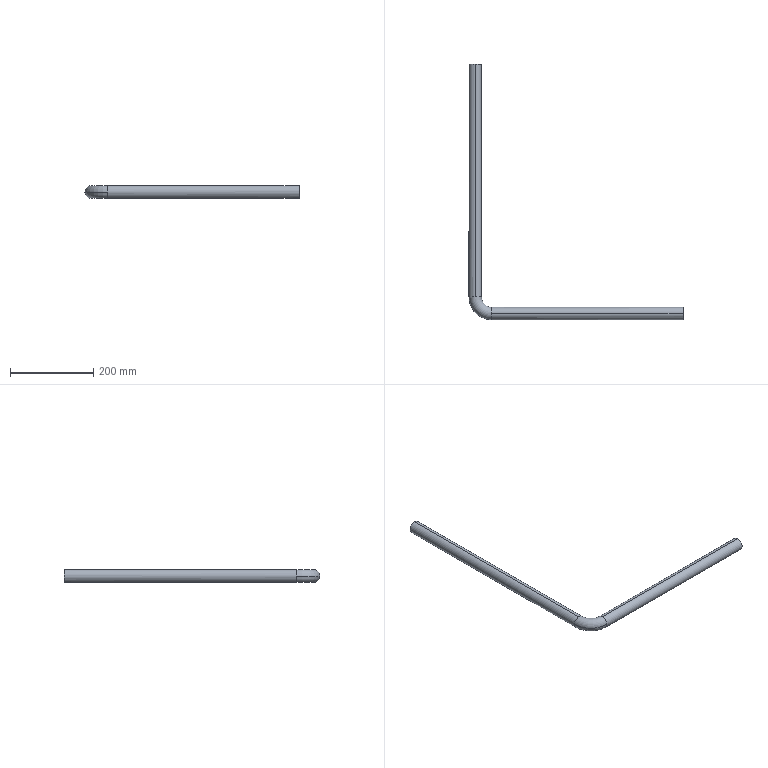Part | SolidWorks | features Sweep 1 | 1 solid | 14 faces | box 515 x 615 x 30 mm | volume 190502 mm3 | cylinder 8 | torus 4 | plane 2 | commonest cylinder face diameters 26 x4 30 x4
STEP:
#1=CARTESIAN_POINT('',(40.,0.,13.));
#2=VERTEX_POINT('',#1);
#3=CARTESIAN_POINT('',(40.,-13.,0.));
#4=VERTEX_POINT('',#3);
#5=CARTESIAN_POINT('',(40.,0.,0.));
#6=DIRECTION('',(1.,0.,0.));
#7=DIRECTION('',(0.,0.,1.));
#8=AXIS2_PLACEMENT_3D('',#5,#6,#7);
#9=CIRCLE('',#8,13.);
#10=EDGE_CURVE('',#2,#4,#9,.T.);
#11=ORIENTED_EDGE('',*,*,#10,.T.);
#12=CARTESIAN_POINT('',(-13.,40.,0.));
#13=VERTEX_POINT('',#12);
#14=CARTESIAN_POINT('',(40.,40.,0.));
#15=DIRECTION('',(0.,0.,-1.));
#16=DIRECTION('',(-1.,0.,0.));
#17=AXIS2_PLACEMENT_3D('',#14,#15,#16);
#18=CIRCLE('',#17,53.);
#19=EDGE_CURVE('',#4,#13,#18,.T.);
#20=ORIENTED_EDGE('',*,*,#19,.T.);
#21=CARTESIAN_POINT('',(0.,40.,13.));
#22=VERTEX_POINT('',#21);
#23=CARTESIAN_POINT('',(0.,40.,0.));
#24=DIRECTION('',(0.,-1.,0.));
#25=DIRECTION('',(1.,0.,0.));
#26=AXIS2_PLACEMENT_3D('',#23,#24,#25);
#27=CIRCLE('',#26,13.);
#28=EDGE_CURVE('',#22,#13,#27,.T.);
#29=ORIENTED_EDGE('',*,*,#28,.F.);
#30=CARTESIAN_POINT('',(13.,40.,0.));
#31=VERTEX_POINT('',#30);
#32=CARTESIAN_POINT('',(0.,40.,0.));
#33=DIRECTION('',(0.,-1.,0.));
#34=DIRECTION('',(1.,0.,0.));
#35=AXIS2_PLACEMENT_3D('',#32,#33,#34);
#36=CIRCLE('',#35,13.);
#37=EDGE_CURVE('',#31,#22,#36,.T.);
#38=ORIENTED_EDGE('',*,*,#37,.F.);
#39=CARTESIAN_POINT('',(40.,13.,0.));
#40=VERTEX_POINT('',#39);
#41=CARTESIAN_POINT('',(40.,40.,0.));
#42=DIRECTION('',(0.,0.,-1.));
#43=DIRECTION('',(-1.,0.,0.));
#44=AXIS2_PLACEMENT_3D('',#41,#42,#43);
#45=CIRCLE('',#44,27.);
#46=EDGE_CURVE('',#40,#31,#45,.T.);
#47=ORIENTED_EDGE('',*,*,#46,.F.);
#48=CARTESIAN_POINT('',(40.,0.,0.));
#49=DIRECTION('',(1.,0.,0.));
#50=DIRECTION('',(0.,0.,1.));
#51=AXIS2_PLACEMENT_3D('',#48,#49,#50);
#52=CIRCLE('',#51,13.);
#53=EDGE_CURVE('',#40,#2,#52,.T.);
#54=ORIENTED_EDGE('',*,*,#53,.T.);
#55=EDGE_LOOP('',(#11,#20,#29,#38,#47,#54));
#56=FACE_OUTER_BOUND('',#55,.T.);
#57=CARTESIAN_POINT('',(40.,40.,0.));
#58=DIRECTION('',(0.,0.,-1.));
#59=DIRECTION('',(-1.,0.,0.));
#60=AXIS2_PLACEMENT_3D('',#57,#58,#59);
#61=TOROIDAL_SURFACE('',#60,40.,13.);
#62=ADVANCED_FACE('',(#56),#61,.F.);
#63=CARTESIAN_POINT('',(40.,-15.,0.));
#64=VERTEX_POINT('',#63);
#65=CARTESIAN_POINT('',(40.,0.,-15.));
#66=VERTEX_POINT('',#65);
#67=CARTESIAN_POINT('',(40.,0.,0.));
#68=DIRECTION('',(1.,0.,0.));
#69=DIRECTION('',(0.,0.,-1.));
#70=AXIS2_PLACEMENT_3D('',#67,#68,#69);
#71=CIRCLE('',#70,15.);
#72=EDGE_CURVE('',#64,#66,#71,.T.);
#73=ORIENTED_EDGE('',*,*,#72,.F.);
#74=CARTESIAN_POINT('',(-15.,40.,0.));
#75=VERTEX_POINT('',#74);
#76=CARTESIAN_POINT('',(40.,40.,0.));
#77=DIRECTION('',(0.,0.,-1.));
#78=DIRECTION('',(-1.,0.,0.));
#79=AXIS2_PLACEMENT_3D('',#76,#77,#78);
#80=CIRCLE('',#79,55.);
#81=EDGE_CURVE('',#64,#75,#80,.T.);
#82=ORIENTED_EDGE('',*,*,#81,.T.);
#83=CARTESIAN_POINT('',(0.,40.,-15.));
#84=VERTEX_POINT('',#83);
#85=CARTESIAN_POINT('',(0.,40.,0.));
#86=DIRECTION('',(0.,-1.,0.));
#87=DIRECTION('',(0.,0.,-1.));
#88=AXIS2_PLACEMENT_3D('',#85,#86,#87);
#89=CIRCLE('',#88,15.);
#90=EDGE_CURVE('',#75,#84,#89,.T.);
#91=ORIENTED_EDGE('',*,*,#90,.T.);
#92=CARTESIAN_POINT('',(15.,40.,0.));
#93=VERTEX_POINT('',#92);
#94=CARTESIAN_POINT('',(0.,40.,0.));
#95=DIRECTION('',(0.,-1.,0.));
#96=DIRECTION('',(0.,0.,-1.));
#97=AXIS2_PLACEMENT_3D('',#94,#95,#96);
#98=CIRCLE('',#97,15.);
#99=EDGE_CURVE('',#84,#93,#98,.T.);
#100=ORIENTED_EDGE('',*,*,#99,.T.);
#101=CARTESIAN_POINT('',(40.,15.,0.));
#102=VERTEX_POINT('',#101);
#103=CARTESIAN_POINT('',(40.,40.,0.));
#104=DIRECTION('',(0.,0.,-1.));
#105=DIRECTION('',(-1.,0.,0.));
#106=AXIS2_PLACEMENT_3D('',#103,#104,#105);
#107=CIRCLE('',#106,25.);
#108=EDGE_CURVE('',#102,#93,#107,.T.);
#109=ORIENTED_EDGE('',*,*,#108,.F.);
#110=CARTESIAN_POINT('',(40.,0.,0.));
#111=DIRECTION('',(1.,0.,0.));
#112=DIRECTION('',(0.,0.,-1.));
#113=AXIS2_PLACEMENT_3D('',#110,#111,#112);
#114=CIRCLE('',#113,15.);
#115=EDGE_CURVE('',#66,#102,#114,.T.);
#116=ORIENTED_EDGE('',*,*,#115,.F.);
#117=EDGE_LOOP('',(#73,#82,#91,#100,#109,#116));
#118=FACE_OUTER_BOUND('',#117,.T.);
#119=CARTESIAN_POINT('',(40.,40.,0.));
#120=DIRECTION('',(0.,0.,-1.));
#121=DIRECTION('',(-1.,0.,0.));
#122=AXIS2_PLACEMENT_3D('',#119,#120,#121);
#123=TOROIDAL_SURFACE('',#122,40.,15.);
#124=ADVANCED_FACE('',(#118),#123,.T.);
#125=ORIENTED_EDGE('',*,*,#28,.T.);
#126=CARTESIAN_POINT('',(0.,40.,-13.));
#127=VERTEX_POINT('',#126);
#128=CARTESIAN_POINT('',(0.,40.,0.));
#129=DIRECTION('',(0.,-1.,0.));
#130=DIRECTION('',(1.,0.,0.));
#131=AXIS2_PLACEMENT_3D('',#128,#129,#130);
#132=CIRCLE('',#131,13.);
#133=EDGE_CURVE('',#13,#127,#132,.T.);
#134=ORIENTED_EDGE('',*,*,#133,.T.);
#135=CARTESIAN_POINT('',(0.,600.,-13.));
#136=VERTEX_POINT('',#135);
#137=CARTESIAN_POINT('',(0.,40.,-13.));
#138=DIRECTION('',(0.,1.,0.));
#139=VECTOR('',#138,1000.);
#140=LINE('',#137,#139);
#141=EDGE_CURVE('',#127,#136,#140,.T.);
#142=ORIENTED_EDGE('',*,*,#141,.T.);
#143=CARTESIAN_POINT('',(0.,600.,13.));
#144=VERTEX_POINT('',#143);
#145=CARTESIAN_POINT('',(0.,600.,0.));
#146=DIRECTION('',(0.,-1.,0.));
#147=DIRECTION('',(0.,0.,-1.));
#148=AXIS2_PLACEMENT_3D('',#145,#146,#147);
#149=CIRCLE('',#148,13.);
#150=EDGE_CURVE('',#144,#136,#149,.T.);
#151=ORIENTED_EDGE('',*,*,#150,.F.);
#152=CARTESIAN_POINT('',(0.,40.,13.));
#153=DIRECTION('',(0.,1.,0.));
#154=VECTOR('',#153,1000.);
#155=LINE('',#152,#154);
#156=EDGE_CURVE('',#22,#144,#155,.T.);
#157=ORIENTED_EDGE('',*,*,#156,.F.);
#158=EDGE_LOOP('',(#125,#134,#142,#151,#157));
#159=FACE_OUTER_BOUND('',#158,.T.);
#160=CARTESIAN_POINT('',(0.,40.,0.));
#161=DIRECTION('',(0.,1.,0.));
#162=DIRECTION('',(0.,0.,1.));
#163=AXIS2_PLACEMENT_3D('',#160,#161,#162);
#164=CYLINDRICAL_SURFACE('',#163,13.);
#165=ADVANCED_FACE('',(#159),#164,.F.);
#166=CARTESIAN_POINT('',(500.,0.,13.));
#167=VERTEX_POINT('',#166);
#168=CARTESIAN_POINT('',(500.,0.,-13.));
#169=VERTEX_POINT('',#168);
#170=CARTESIAN_POINT('',(500.,0.,0.));
#171=DIRECTION('',(1.,0.,0.));
#172=DIRECTION('',(0.,0.,-1.));
#173=AXIS2_PLACEMENT_3D('',#170,#171,#172);
#174=CIRCLE('',#173,13.);
#175=EDGE_CURVE('',#167,#169,#174,.T.);
#176=ORIENTED_EDGE('',*,*,#175,.T.);
#177=CARTESIAN_POINT('',(40.,0.,-13.));
#178=VERTEX_POINT('',#177);
#179=CARTESIAN_POINT('',(500.,0.,-13.));
#180=DIRECTION('',(-1.,0.,0.));
#181=VECTOR('',#180,1000.);
#182=LINE('',#179,#181);
#183=EDGE_CURVE('',#169,#178,#182,.T.);
#184=ORIENTED_EDGE('',*,*,#183,.T.);
#185=CARTESIAN_POINT('',(40.,0.,0.));
#186=DIRECTION('',(1.,0.,0.));
#187=DIRECTION('',(0.,0.,1.));
#188=AXIS2_PLACEMENT_3D('',#185,#186,#187);
#189=CIRCLE('',#188,13.);
#190=EDGE_CURVE('',#4,#178,#189,.T.);
#191=ORIENTED_EDGE('',*,*,#190,.F.);
#192=ORIENTED_EDGE('',*,*,#10,.F.);
#193=CARTESIAN_POINT('',(500.,0.,13.));
#194=DIRECTION('',(-1.,0.,0.));
#195=VECTOR('',#194,1000.);
#196=LINE('',#193,#195);
#197=EDGE_CURVE('',#167,#2,#196,.T.);
#198=ORIENTED_EDGE('',*,*,#197,.F.);
#199=EDGE_LOOP('',(#176,#184,#191,#192,#198));
#200=FACE_OUTER_BOUND('',#199,.T.);
#201=CARTESIAN_POINT('',(500.,0.,0.));
#202=DIRECTION('',(-1.,0.,0.));
#203=DIRECTION('',(0.,0.,1.));
#204=AXIS2_PLACEMENT_3D('',#201,#202,#203);
#205=CYLINDRICAL_SURFACE('',#204,13.);
#206=ADVANCED_FACE('',(#200),#205,.F.);
#207=ORIENTED_EDGE('',*,*,#99,.F.);
#208=CARTESIAN_POINT('',(0.,600.,-15.));
#209=VERTEX_POINT('',#208);
#210=CARTESIAN_POINT('',(0.,40.,-15.));
#211=DIRECTION('',(0.,1.,0.));
#212=VECTOR('',#211,1000.);
#213=LINE('',#210,#212);
#214=EDGE_CURVE('',#84,#209,#213,.T.);
#215=ORIENTED_EDGE('',*,*,#214,.T.);
#216=CARTESIAN_POINT('',(0.,600.,15.));
#217=VERTEX_POINT('',#216);
#218=CARTESIAN_POINT('',(0.,600.,0.));
#219=DIRECTION('',(0.,-1.,0.));
#220=DIRECTION('',(0.,0.,-1.));
#221=AXIS2_PLACEMENT_3D('',#218,#219,#220);
#222=CIRCLE('',#221,15.);
#223=EDGE_CURVE('',#209,#217,#222,.T.);
#224=ORIENTED_EDGE('',*,*,#223,.T.);
#225=CARTESIAN_POINT('',(0.,40.,15.));
#226=VERTEX_POINT('',#225);
#227=CARTESIAN_POINT('',(0.,40.,15.));
#228=DIRECTION('',(0.,1.,0.));
#229=VECTOR('',#228,1000.);
#230=LINE('',#227,#229);
#231=EDGE_CURVE('',#226,#217,#230,.T.);
#232=ORIENTED_EDGE('',*,*,#231,.F.);
#233=CARTESIAN_POINT('',(0.,40.,0.));
#234=DIRECTION('',(0.,-1.,0.));
#235=DIRECTION('',(0.,0.,-1.));
#236=AXIS2_PLACEMENT_3D('',#233,#234,#235);
#237=CIRCLE('',#236,15.);
#238=EDGE_CURVE('',#93,#226,#237,.T.);
#239=ORIENTED_EDGE('',*,*,#238,.F.);
#240=EDGE_LOOP('',(#207,#215,#224,#232,#239));
#241=FACE_OUTER_BOUND('',#240,.T.);
#242=CARTESIAN_POINT('',(0.,40.,0.));
#243=DIRECTION('',(0.,1.,0.));
#244=DIRECTION('',(0.,0.,1.));
#245=AXIS2_PLACEMENT_3D('',#242,#243,#244);
#246=CYLINDRICAL_SURFACE('',#245,15.);
#247=ADVANCED_FACE('',(#241),#246,.T.);
#248=CARTESIAN_POINT('',(500.,0.,-15.));
#249=VERTEX_POINT('',#248);
#250=CARTESIAN_POINT('',(500.,0.,15.));
#251=VERTEX_POINT('',#250);
#252=CARTESIAN_POINT('',(500.,0.,0.));
#253=DIRECTION('',(1.,0.,0.));
#254=DIRECTION('',(0.,0.,-1.));
#255=AXIS2_PLACEMENT_3D('',#252,#253,#254);
#256=CIRCLE('',#255,15.);
#257=EDGE_CURVE('',#249,#251,#256,.T.);
#258=ORIENTED_EDGE('',*,*,#257,.F.);
#259=CARTESIAN_POINT('',(500.,0.,-15.));
#260=DIRECTION('',(-1.,0.,0.));
#261=VECTOR('',#260,1000.);
#262=LINE('',#259,#261);
#263=EDGE_CURVE('',#249,#66,#262,.T.);
#264=ORIENTED_EDGE('',*,*,#263,.T.);
#265=ORIENTED_EDGE('',*,*,#115,.T.);
#266=CARTESIAN_POINT('',(40.,0.,15.));
#267=VERTEX_POINT('',#266);
#268=CARTESIAN_POINT('',(40.,0.,0.));
#269=DIRECTION('',(1.,0.,0.));
#270=DIRECTION('',(0.,0.,-1.));
#271=AXIS2_PLACEMENT_3D('',#268,#269,#270);
#272=CIRCLE('',#271,15.);
#273=EDGE_CURVE('',#102,#267,#272,.T.);
#274=ORIENTED_EDGE('',*,*,#273,.T.);
#275=CARTESIAN_POINT('',(500.,0.,15.));
#276=DIRECTION('',(-1.,0.,0.));
#277=VECTOR('',#276,1000.);
#278=LINE('',#275,#277);
#279=EDGE_CURVE('',#251,#267,#278,.T.);
#280=ORIENTED_EDGE('',*,*,#279,.F.);
#281=EDGE_LOOP('',(#258,#264,#265,#274,#280));
#282=FACE_OUTER_BOUND('',#281,.T.);
#283=CARTESIAN_POINT('',(500.,0.,0.));
#284=DIRECTION('',(-1.,0.,0.));
#285=DIRECTION('',(0.,0.,1.));
#286=AXIS2_PLACEMENT_3D('',#283,#284,#285);
#287=CYLINDRICAL_SURFACE('',#286,15.);
#288=ADVANCED_FACE('',(#282),#287,.T.);
#289=ORIENTED_EDGE('',*,*,#214,.F.);
#290=ORIENTED_EDGE('',*,*,#90,.F.);
#291=CARTESIAN_POINT('',(0.,40.,0.));
#292=DIRECTION('',(0.,-1.,0.));
#293=DIRECTION('',(0.,0.,-1.));
#294=AXIS2_PLACEMENT_3D('',#291,#292,#293);
#295=CIRCLE('',#294,15.);
#296=EDGE_CURVE('',#226,#75,#295,.T.);
#297=ORIENTED_EDGE('',*,*,#296,.F.);
#298=ORIENTED_EDGE('',*,*,#231,.T.);
#299=CARTESIAN_POINT('',(0.,600.,0.));
#300=DIRECTION('',(0.,-1.,0.));
#301=DIRECTION('',(0.,0.,-1.));
#302=AXIS2_PLACEMENT_3D('',#299,#300,#301);
#303=CIRCLE('',#302,15.);
#304=EDGE_CURVE('',#217,#209,#303,.T.);
#305=ORIENTED_EDGE('',*,*,#304,.T.);
#306=EDGE_LOOP('',(#289,#290,#297,#298,#305));
#307=FACE_OUTER_BOUND('',#306,.T.);
#308=CARTESIAN_POINT('',(0.,40.,0.));
#309=DIRECTION('',(0.,1.,0.));
#310=DIRECTION('',(0.,0.,1.));
#311=AXIS2_PLACEMENT_3D('',#308,#309,#310);
#312=CYLINDRICAL_SURFACE('',#311,15.);
#313=ADVANCED_FACE('',(#307),#312,.T.);
#314=ORIENTED_EDGE('',*,*,#81,.F.);
#315=CARTESIAN_POINT('',(40.,0.,0.));
#316=DIRECTION('',(1.,0.,0.));
#317=DIRECTION('',(0.,0.,-1.));
#318=AXIS2_PLACEMENT_3D('',#315,#316,#317);
#319=CIRCLE('',#318,15.);
#320=EDGE_CURVE('',#267,#64,#319,.T.);
#321=ORIENTED_EDGE('',*,*,#320,.F.);
#322=ORIENTED_EDGE('',*,*,#273,.F.);
#323=ORIENTED_EDGE('',*,*,#108,.T.);
#324=ORIENTED_EDGE('',*,*,#238,.T.);
#325=ORIENTED_EDGE('',*,*,#296,.T.);
#326=EDGE_LOOP('',(#314,#321,#322,#323,#324,#325));
#327=FACE_OUTER_BOUND('',#326,.T.);
#328=CARTESIAN_POINT('',(40.,40.,0.));
#329=DIRECTION('',(0.,0.,-1.));
#330=DIRECTION('',(-1.,0.,0.));
#331=AXIS2_PLACEMENT_3D('',#328,#329,#330);
#332=TOROIDAL_SURFACE('',#331,40.,15.);
#333=ADVANCED_FACE('',(#327),#332,.T.);
#334=ORIENTED_EDGE('',*,*,#263,.F.);
#335=CARTESIAN_POINT('',(500.,0.,0.));
#336=DIRECTION('',(1.,0.,0.));
#337=DIRECTION('',(0.,0.,-1.));
#338=AXIS2_PLACEMENT_3D('',#335,#336,#337);
#339=CIRCLE('',#338,15.);
#340=EDGE_CURVE('',#251,#249,#339,.T.);
#341=ORIENTED_EDGE('',*,*,#340,.F.);
#342=ORIENTED_EDGE('',*,*,#279,.T.);
#343=ORIENTED_EDGE('',*,*,#320,.T.);
#344=ORIENTED_EDGE('',*,*,#72,.T.);
#345=EDGE_LOOP('',(#334,#341,#342,#343,#344));
#346=FACE_OUTER_BOUND('',#345,.T.);
#347=CARTESIAN_POINT('',(500.,0.,0.));
#348=DIRECTION('',(-1.,0.,0.));
#349=DIRECTION('',(0.,0.,1.));
#350=AXIS2_PLACEMENT_3D('',#347,#348,#349);
#351=CYLINDRICAL_SURFACE('',#350,15.);
#352=ADVANCED_FACE('',(#346),#351,.T.);
#353=ORIENTED_EDGE('',*,*,#150,.T.);
#354=CARTESIAN_POINT('',(0.,600.,0.));
#355=DIRECTION('',(0.,-1.,0.));
#356=DIRECTION('',(0.,0.,-1.));
#357=AXIS2_PLACEMENT_3D('',#354,#355,#356);
#358=CIRCLE('',#357,13.);
#359=EDGE_CURVE('',#136,#144,#358,.T.);
#360=ORIENTED_EDGE('',*,*,#359,.T.);
#361=EDGE_LOOP('',(#353,#360));
#362=FACE_BOUND('',#361,.T.);
#363=ORIENTED_EDGE('',*,*,#304,.F.);
#364=ORIENTED_EDGE('',*,*,#223,.F.);
#365=EDGE_LOOP('',(#363,#364));
#366=FACE_OUTER_BOUND('',#365,.T.);
#367=CARTESIAN_POINT('',(0.,600.,0.));
#368=DIRECTION('',(0.,-1.,0.));
#369=DIRECTION('',(0.,0.,-1.));
#370=AXIS2_PLACEMENT_3D('',#367,#368,#369);
#371=PLANE('',#370);
#372=ADVANCED_FACE('',(#362,#366),#371,.F.);
#373=ORIENTED_EDGE('',*,*,#175,.F.);
#374=CARTESIAN_POINT('',(500.,0.,0.));
#375=DIRECTION('',(1.,0.,0.));
#376=DIRECTION('',(0.,0.,-1.));
#377=AXIS2_PLACEMENT_3D('',#374,#375,#376);
#378=CIRCLE('',#377,13.);
#379=EDGE_CURVE('',#169,#167,#378,.T.);
#380=ORIENTED_EDGE('',*,*,#379,.F.);
#381=EDGE_LOOP('',(#373,#380));
#382=FACE_BOUND('',#381,.T.);
#383=ORIENTED_EDGE('',*,*,#340,.T.);
#384=ORIENTED_EDGE('',*,*,#257,.T.);
#385=EDGE_LOOP('',(#383,#384));
#386=FACE_OUTER_BOUND('',#385,.T.);
#387=CARTESIAN_POINT('',(500.,0.,0.));
#388=DIRECTION('',(1.,0.,0.));
#389=DIRECTION('',(0.,0.,-1.));
#390=AXIS2_PLACEMENT_3D('',#387,#388,#389);
#391=PLANE('',#390);
#392=ADVANCED_FACE('',(#382,#386),#391,.T.);
#393=ORIENTED_EDGE('',*,*,#141,.F.);
#394=CARTESIAN_POINT('',(0.,40.,0.));
#395=DIRECTION('',(0.,-1.,0.));
#396=DIRECTION('',(1.,0.,0.));
#397=AXIS2_PLACEMENT_3D('',#394,#395,#396);
#398=CIRCLE('',#397,13.);
#399=EDGE_CURVE('',#127,#31,#398,.T.);
#400=ORIENTED_EDGE('',*,*,#399,.T.);
#401=ORIENTED_EDGE('',*,*,#37,.T.);
#402=ORIENTED_EDGE('',*,*,#156,.T.);
#403=ORIENTED_EDGE('',*,*,#359,.F.);
#404=EDGE_LOOP('',(#393,#400,#401,#402,#403));
#405=FACE_OUTER_BOUND('',#404,.T.);
#406=CARTESIAN_POINT('',(0.,40.,0.));
#407=DIRECTION('',(0.,1.,0.));
#408=DIRECTION('',(0.,0.,1.));
#409=AXIS2_PLACEMENT_3D('',#406,#407,#408);
#410=CYLINDRICAL_SURFACE('',#409,13.);
#411=ADVANCED_FACE('',(#405),#410,.F.);
#412=ORIENTED_EDGE('',*,*,#19,.F.);
#413=ORIENTED_EDGE('',*,*,#190,.T.);
#414=CARTESIAN_POINT('',(40.,0.,0.));
#415=DIRECTION('',(1.,0.,0.));
#416=DIRECTION('',(0.,0.,1.));
#417=AXIS2_PLACEMENT_3D('',#414,#415,#416);
#418=CIRCLE('',#417,13.);
#419=EDGE_CURVE('',#178,#40,#418,.T.);
#420=ORIENTED_EDGE('',*,*,#419,.T.);
#421=ORIENTED_EDGE('',*,*,#46,.T.);
#422=ORIENTED_EDGE('',*,*,#399,.F.);
#423=ORIENTED_EDGE('',*,*,#133,.F.);
#424=EDGE_LOOP('',(#412,#413,#420,#421,#422,#423));
#425=FACE_OUTER_BOUND('',#424,.T.);
#426=CARTESIAN_POINT('',(40.,40.,0.));
#427=DIRECTION('',(0.,0.,-1.));
#428=DIRECTION('',(-1.,0.,0.));
#429=AXIS2_PLACEMENT_3D('',#426,#427,#428);
#430=TOROIDAL_SURFACE('',#429,40.,13.);
#431=ADVANCED_FACE('',(#425),#430,.F.);
#432=ORIENTED_EDGE('',*,*,#183,.F.);
#433=ORIENTED_EDGE('',*,*,#379,.T.);
#434=ORIENTED_EDGE('',*,*,#197,.T.);
#435=ORIENTED_EDGE('',*,*,#53,.F.);
#436=ORIENTED_EDGE('',*,*,#419,.F.);
#437=EDGE_LOOP('',(#432,#433,#434,#435,#436));
#438=FACE_OUTER_BOUND('',#437,.T.);
#439=CARTESIAN_POINT('',(500.,0.,0.));
#440=DIRECTION('',(-1.,0.,0.));
#441=DIRECTION('',(0.,0.,1.));
#442=AXIS2_PLACEMENT_3D('',#439,#440,#441);
#443=CYLINDRICAL_SURFACE('',#442,13.);
#444=ADVANCED_FACE('',(#438),#443,.F.);
#445=CLOSED_SHELL('',(#62,#124,#165,#206,#247,#288,#313,#333,#352,#372,#392,#411,#431,#444));
#446=MANIFOLD_SOLID_BREP('',#445);
#447=CARTESIAN_POINT('',(0.,0.,0.));
#448=DIRECTION('',(0.,0.,1.));
#449=DIRECTION('',(1.,0.,0.));
#450=AXIS2_PLACEMENT_3D('',#447,#448,#449);
#451=(LENGTH_UNIT()NAMED_UNIT(*)SI_UNIT(.MILLI.,.METRE.));
#452=UNCERTAINTY_MEASURE_WITH_UNIT(LENGTH_MEASURE(0.00001),#451,'','');
#453=(NAMED_UNIT(*)PLANE_ANGLE_UNIT()SI_UNIT($,.RADIAN.));
#454=(NAMED_UNIT(*)SI_UNIT($,.STERADIAN.)SOLID_ANGLE_UNIT());
#455=(GEOMETRIC_REPRESENTATION_CONTEXT(3)GLOBAL_UNCERTAINTY_ASSIGNED_CONTEXT((#452))GLOBAL_UNIT_ASSIGNED_CONTEXT((#451,#453,#454))REPRESENTATION_CONTEXT('',''));
#456=ADVANCED_BREP_SHAPE_REPRESENTATION('',(#446,#450),#455);